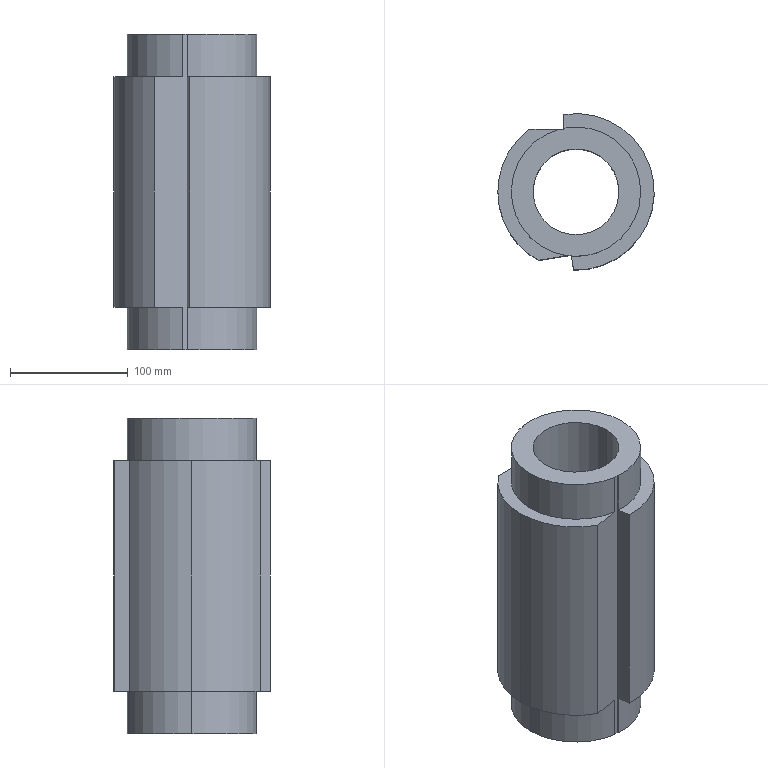Part | SolidWorks | features ICE 2, Extrusion 1 | 1 solid | 21 faces | box 133 x 133 x 268 mm | volume 2196545 mm3 | cylinder 11 | plane 10 | commonest cylinder face diameters 110 x6 133 x3 73 x2
STEP:
#1=CARTESIAN_POINT('',(-7.929,-54.426,36.));
#2=VERTEX_POINT('',#1);
#3=CARTESIAN_POINT('',(-55.,0.,36.));
#4=VERTEX_POINT('',#3);
#5=CARTESIAN_POINT('',(0.,0.,36.));
#6=DIRECTION('',(0.,0.,-1.));
#7=DIRECTION('',(-1.,0.,0.));
#8=AXIS2_PLACEMENT_3D('',#5,#6,#7);
#9=CIRCLE('',#8,55.);
#10=EDGE_CURVE('',#2,#4,#9,.T.);
#11=ORIENTED_EDGE('',*,*,#10,.T.);
#12=CARTESIAN_POINT('',(-55.,0.,0.));
#13=VERTEX_POINT('',#12);
#14=CARTESIAN_POINT('',(-55.,0.,36.));
#15=DIRECTION('',(0.,0.,-1.));
#16=VECTOR('',#15,1000.);
#17=LINE('',#14,#16);
#18=EDGE_CURVE('',#4,#13,#17,.T.);
#19=ORIENTED_EDGE('',*,*,#18,.T.);
#20=CARTESIAN_POINT('',(-7.929,-54.426,0.));
#21=VERTEX_POINT('',#20);
#22=CARTESIAN_POINT('',(0.,0.,0.));
#23=DIRECTION('',(0.,0.,1.));
#24=DIRECTION('',(1.,0.,0.));
#25=AXIS2_PLACEMENT_3D('',#22,#23,#24);
#26=CIRCLE('',#25,55.);
#27=EDGE_CURVE('',#13,#21,#26,.T.);
#28=ORIENTED_EDGE('',*,*,#27,.T.);
#29=CARTESIAN_POINT('',(-7.929,-54.426,36.));
#30=DIRECTION('',(0.,0.,1.));
#31=VECTOR('',#30,1000.);
#32=LINE('',#29,#31);
#33=EDGE_CURVE('',#21,#2,#32,.T.);
#34=ORIENTED_EDGE('',*,*,#33,.T.);
#35=EDGE_LOOP('',(#11,#19,#28,#34));
#36=FACE_OUTER_BOUND('',#35,.T.);
#37=CARTESIAN_POINT('',(0.,0.,36.));
#38=DIRECTION('',(0.,0.,-1.));
#39=DIRECTION('',(-1.,0.,0.));
#40=AXIS2_PLACEMENT_3D('',#37,#38,#39);
#41=CYLINDRICAL_SURFACE('',#40,55.);
#42=ADVANCED_FACE('',(#36),#41,.T.);
#43=CARTESIAN_POINT('',(-3.964,-54.857,232.));
#44=VERTEX_POINT('',#43);
#45=CARTESIAN_POINT('',(55.,0.,232.));
#46=VERTEX_POINT('',#45);
#47=CARTESIAN_POINT('',(0.,0.,232.));
#48=DIRECTION('',(0.,0.,1.));
#49=DIRECTION('',(1.,0.,0.));
#50=AXIS2_PLACEMENT_3D('',#47,#48,#49);
#51=CIRCLE('',#50,55.);
#52=EDGE_CURVE('',#44,#46,#51,.T.);
#53=ORIENTED_EDGE('',*,*,#52,.T.);
#54=CARTESIAN_POINT('',(55.,0.,268.));
#55=VERTEX_POINT('',#54);
#56=CARTESIAN_POINT('',(55.,0.,232.));
#57=DIRECTION('',(0.,0.,1.));
#58=VECTOR('',#57,1000.);
#59=LINE('',#56,#58);
#60=EDGE_CURVE('',#46,#55,#59,.T.);
#61=ORIENTED_EDGE('',*,*,#60,.T.);
#62=CARTESIAN_POINT('',(-3.964,-54.857,268.));
#63=VERTEX_POINT('',#62);
#64=CARTESIAN_POINT('',(0.,0.,268.));
#65=DIRECTION('',(0.,0.,1.));
#66=DIRECTION('',(1.,0.,0.));
#67=AXIS2_PLACEMENT_3D('',#64,#65,#66);
#68=CIRCLE('',#67,55.);
#69=EDGE_CURVE('',#63,#55,#68,.T.);
#70=ORIENTED_EDGE('',*,*,#69,.F.);
#71=CARTESIAN_POINT('',(-3.964,-54.857,232.));
#72=DIRECTION('',(0.,0.,-1.));
#73=VECTOR('',#72,1000.);
#74=LINE('',#71,#73);
#75=EDGE_CURVE('',#63,#44,#74,.T.);
#76=ORIENTED_EDGE('',*,*,#75,.T.);
#77=EDGE_LOOP('',(#53,#61,#70,#76));
#78=FACE_OUTER_BOUND('',#77,.T.);
#79=CARTESIAN_POINT('',(0.,0.,232.));
#80=DIRECTION('',(0.,0.,1.));
#81=DIRECTION('',(1.,0.,0.));
#82=AXIS2_PLACEMENT_3D('',#79,#80,#81);
#83=CYLINDRICAL_SURFACE('',#82,55.);
#84=ADVANCED_FACE('',(#78),#83,.T.);
#85=CARTESIAN_POINT('',(-36.5,0.,268.));
#86=VERTEX_POINT('',#85);
#87=CARTESIAN_POINT('',(36.5,0.,268.));
#88=VERTEX_POINT('',#87);
#89=CARTESIAN_POINT('',(0.,0.,268.));
#90=DIRECTION('',(0.,0.,1.));
#91=DIRECTION('',(1.,0.,0.));
#92=AXIS2_PLACEMENT_3D('',#89,#90,#91);
#93=CIRCLE('',#92,36.5);
#94=EDGE_CURVE('',#86,#88,#93,.T.);
#95=ORIENTED_EDGE('',*,*,#94,.T.);
#96=CARTESIAN_POINT('',(36.5,0.,0.));
#97=VERTEX_POINT('',#96);
#98=CARTESIAN_POINT('',(36.5,0.,268.));
#99=DIRECTION('',(0.,0.,-1.));
#100=VECTOR('',#99,1000.);
#101=LINE('',#98,#100);
#102=EDGE_CURVE('',#88,#97,#101,.T.);
#103=ORIENTED_EDGE('',*,*,#102,.T.);
#104=CARTESIAN_POINT('',(-36.5,0.,0.));
#105=VERTEX_POINT('',#104);
#106=CARTESIAN_POINT('',(0.,0.,0.));
#107=DIRECTION('',(0.,0.,1.));
#108=DIRECTION('',(1.,0.,0.));
#109=AXIS2_PLACEMENT_3D('',#106,#107,#108);
#110=CIRCLE('',#109,36.5);
#111=EDGE_CURVE('',#105,#97,#110,.T.);
#112=ORIENTED_EDGE('',*,*,#111,.F.);
#113=CARTESIAN_POINT('',(-36.5,0.,268.));
#114=DIRECTION('',(0.,0.,-1.));
#115=VECTOR('',#114,1000.);
#116=LINE('',#113,#115);
#117=EDGE_CURVE('',#86,#105,#116,.T.);
#118=ORIENTED_EDGE('',*,*,#117,.F.);
#119=EDGE_LOOP('',(#95,#103,#112,#118));
#120=FACE_OUTER_BOUND('',#119,.T.);
#121=CARTESIAN_POINT('',(0.,0.,268.));
#122=DIRECTION('',(0.,0.,-1.));
#123=DIRECTION('',(-1.,0.,0.));
#124=AXIS2_PLACEMENT_3D('',#121,#122,#123);
#125=CYLINDRICAL_SURFACE('',#124,36.5);
#126=ADVANCED_FACE('',(#120),#125,.F.);
#127=CARTESIAN_POINT('',(-66.5,0.,232.));
#128=VERTEX_POINT('',#127);
#129=CARTESIAN_POINT('',(-32.08,-58.251,232.));
#130=VERTEX_POINT('',#129);
#131=CARTESIAN_POINT('',(0.,0.,232.));
#132=DIRECTION('',(0.,0.,1.));
#133=DIRECTION('',(1.,0.,0.));
#134=AXIS2_PLACEMENT_3D('',#131,#132,#133);
#135=CIRCLE('',#134,66.5);
#136=EDGE_CURVE('',#128,#130,#135,.T.);
#137=ORIENTED_EDGE('',*,*,#136,.F.);
#138=CARTESIAN_POINT('',(-66.5,0.,36.));
#139=VERTEX_POINT('',#138);
#140=CARTESIAN_POINT('',(-66.5,0.,268.));
#141=DIRECTION('',(0.,0.,-1.));
#142=VECTOR('',#141,1000.);
#143=LINE('',#140,#142);
#144=EDGE_CURVE('',#128,#139,#143,.T.);
#145=ORIENTED_EDGE('',*,*,#144,.T.);
#146=CARTESIAN_POINT('',(-32.08,-58.251,36.));
#147=VERTEX_POINT('',#146);
#148=CARTESIAN_POINT('',(0.,0.,36.));
#149=DIRECTION('',(0.,0.,-1.));
#150=DIRECTION('',(-1.,0.,0.));
#151=AXIS2_PLACEMENT_3D('',#148,#149,#150);
#152=CIRCLE('',#151,66.5);
#153=EDGE_CURVE('',#147,#139,#152,.T.);
#154=ORIENTED_EDGE('',*,*,#153,.F.);
#155=CARTESIAN_POINT('',(-32.08,-58.251,268.));
#156=DIRECTION('',(0.,0.,-1.));
#157=VECTOR('',#156,1000.);
#158=LINE('',#155,#157);
#159=EDGE_CURVE('',#130,#147,#158,.T.);
#160=ORIENTED_EDGE('',*,*,#159,.F.);
#161=EDGE_LOOP('',(#137,#145,#154,#160));
#162=FACE_OUTER_BOUND('',#161,.T.);
#163=CARTESIAN_POINT('',(0.,0.,268.));
#164=DIRECTION('',(0.,0.,-1.));
#165=DIRECTION('',(-1.,0.,0.));
#166=AXIS2_PLACEMENT_3D('',#163,#164,#165);
#167=CYLINDRICAL_SURFACE('',#166,66.5);
#168=ADVANCED_FACE('',(#162),#167,.T.);
#169=CARTESIAN_POINT('',(-4.128,-53.824,36.));
#170=DIRECTION('',(-0.9877,-0.1564,0.));
#171=VECTOR('',#170,1000.);
#172=LINE('',#169,#171);
#173=EDGE_CURVE('',#2,#147,#172,.T.);
#174=ORIENTED_EDGE('',*,*,#173,.F.);
#175=ORIENTED_EDGE('',*,*,#33,.F.);
#176=CARTESIAN_POINT('',(-4.128,-53.824,0.));
#177=VERTEX_POINT('',#176);
#178=CARTESIAN_POINT('',(-4.128,-53.824,0.));
#179=DIRECTION('',(0.9877,0.1564,0.));
#180=VECTOR('',#179,1000.);
#181=LINE('',#178,#180);
#182=EDGE_CURVE('',#21,#177,#181,.T.);
#183=ORIENTED_EDGE('',*,*,#182,.T.);
#184=CARTESIAN_POINT('',(-4.128,-53.824,268.));
#185=VERTEX_POINT('',#184);
#186=CARTESIAN_POINT('',(-4.128,-53.824,268.));
#187=DIRECTION('',(0.,0.,-1.));
#188=VECTOR('',#187,1000.);
#189=LINE('',#186,#188);
#190=EDGE_CURVE('',#185,#177,#189,.T.);
#191=ORIENTED_EDGE('',*,*,#190,.F.);
#192=CARTESIAN_POINT('',(-7.929,-54.426,268.));
#193=VERTEX_POINT('',#192);
#194=CARTESIAN_POINT('',(-4.128,-53.824,268.));
#195=DIRECTION('',(0.9877,0.1564,0.));
#196=VECTOR('',#195,1000.);
#197=LINE('',#194,#196);
#198=EDGE_CURVE('',#193,#185,#197,.T.);
#199=ORIENTED_EDGE('',*,*,#198,.F.);
#200=CARTESIAN_POINT('',(-7.929,-54.426,232.));
#201=VERTEX_POINT('',#200);
#202=CARTESIAN_POINT('',(-7.929,-54.426,232.));
#203=DIRECTION('',(0.,0.,1.));
#204=VECTOR('',#203,1000.);
#205=LINE('',#202,#204);
#206=EDGE_CURVE('',#201,#193,#205,.T.);
#207=ORIENTED_EDGE('',*,*,#206,.F.);
#208=CARTESIAN_POINT('',(-4.128,-53.824,232.));
#209=DIRECTION('',(0.9877,0.1564,0.));
#210=VECTOR('',#209,1000.);
#211=LINE('',#208,#210);
#212=EDGE_CURVE('',#130,#201,#211,.T.);
#213=ORIENTED_EDGE('',*,*,#212,.F.);
#214=ORIENTED_EDGE('',*,*,#159,.T.);
#215=EDGE_LOOP('',(#174,#175,#183,#191,#199,#207,#213,#214));
#216=FACE_OUTER_BOUND('',#215,.T.);
#217=CARTESIAN_POINT('',(-4.128,-53.824,268.));
#218=DIRECTION('',(-0.1564,0.9877,0.));
#219=DIRECTION('',(-0.9877,-0.1564,0.));
#220=AXIS2_PLACEMENT_3D('',#217,#218,#219);
#221=PLANE('',#220);
#222=ADVANCED_FACE('',(#216),#221,.F.);
#223=CARTESIAN_POINT('',(-2.126,-66.466,36.));
#224=VERTEX_POINT('',#223);
#225=CARTESIAN_POINT('',(-3.964,-54.857,36.));
#226=VERTEX_POINT('',#225);
#227=CARTESIAN_POINT('',(-4.128,-53.824,36.));
#228=DIRECTION('',(-0.1564,0.9877,0.));
#229=VECTOR('',#228,1000.);
#230=LINE('',#227,#229);
#231=EDGE_CURVE('',#224,#226,#230,.T.);
#232=ORIENTED_EDGE('',*,*,#231,.F.);
#233=CARTESIAN_POINT('',(-2.126,-66.466,232.));
#234=VERTEX_POINT('',#233);
#235=CARTESIAN_POINT('',(-2.126,-66.466,268.));
#236=DIRECTION('',(0.,0.,-1.));
#237=VECTOR('',#236,1000.);
#238=LINE('',#235,#237);
#239=EDGE_CURVE('',#234,#224,#238,.T.);
#240=ORIENTED_EDGE('',*,*,#239,.F.);
#241=CARTESIAN_POINT('',(-4.128,-53.824,232.));
#242=DIRECTION('',(0.1564,-0.9877,0.));
#243=VECTOR('',#242,1000.);
#244=LINE('',#241,#243);
#245=EDGE_CURVE('',#44,#234,#244,.T.);
#246=ORIENTED_EDGE('',*,*,#245,.F.);
#247=ORIENTED_EDGE('',*,*,#75,.F.);
#248=CARTESIAN_POINT('',(-4.128,-53.824,268.));
#249=DIRECTION('',(0.1564,-0.9877,0.));
#250=VECTOR('',#249,1000.);
#251=LINE('',#248,#250);
#252=EDGE_CURVE('',#185,#63,#251,.T.);
#253=ORIENTED_EDGE('',*,*,#252,.F.);
#254=ORIENTED_EDGE('',*,*,#190,.T.);
#255=CARTESIAN_POINT('',(-3.964,-54.857,0.));
#256=VERTEX_POINT('',#255);
#257=CARTESIAN_POINT('',(-4.128,-53.824,0.));
#258=DIRECTION('',(0.1564,-0.9877,0.));
#259=VECTOR('',#258,1000.);
#260=LINE('',#257,#259);
#261=EDGE_CURVE('',#177,#256,#260,.T.);
#262=ORIENTED_EDGE('',*,*,#261,.T.);
#263=CARTESIAN_POINT('',(-3.964,-54.857,36.));
#264=DIRECTION('',(0.,0.,-1.));
#265=VECTOR('',#264,1000.);
#266=LINE('',#263,#265);
#267=EDGE_CURVE('',#226,#256,#266,.T.);
#268=ORIENTED_EDGE('',*,*,#267,.F.);
#269=EDGE_LOOP('',(#232,#240,#246,#247,#253,#254,#262,#268));
#270=FACE_OUTER_BOUND('',#269,.T.);
#271=CARTESIAN_POINT('',(-4.128,-53.824,268.));
#272=DIRECTION('',(0.9877,0.1564,0.));
#273=DIRECTION('',(-0.1564,0.9877,0.));
#274=AXIS2_PLACEMENT_3D('',#271,#272,#273);
#275=PLANE('',#274);
#276=ADVANCED_FACE('',(#270),#275,.F.);
#277=CARTESIAN_POINT('',(-10.3,65.697,36.));
#278=VERTEX_POINT('',#277);
#279=CARTESIAN_POINT('',(0.,0.,36.));
#280=DIRECTION('',(0.,0.,-1.));
#281=DIRECTION('',(-1.,0.,0.));
#282=AXIS2_PLACEMENT_3D('',#279,#280,#281);
#283=CIRCLE('',#282,66.5);
#284=EDGE_CURVE('',#278,#224,#283,.T.);
#285=ORIENTED_EDGE('',*,*,#284,.F.);
#286=CARTESIAN_POINT('',(-10.3,65.697,232.));
#287=VERTEX_POINT('',#286);
#288=CARTESIAN_POINT('',(-10.3,65.697,268.));
#289=DIRECTION('',(0.,0.,-1.));
#290=VECTOR('',#289,1000.);
#291=LINE('',#288,#290);
#292=EDGE_CURVE('',#287,#278,#291,.T.);
#293=ORIENTED_EDGE('',*,*,#292,.F.);
#294=CARTESIAN_POINT('',(0.,0.,232.));
#295=DIRECTION('',(0.,0.,1.));
#296=DIRECTION('',(1.,0.,0.));
#297=AXIS2_PLACEMENT_3D('',#294,#295,#296);
#298=CIRCLE('',#297,66.5);
#299=EDGE_CURVE('',#234,#287,#298,.T.);
#300=ORIENTED_EDGE('',*,*,#299,.F.);
#301=ORIENTED_EDGE('',*,*,#239,.T.);
#302=EDGE_LOOP('',(#285,#293,#300,#301));
#303=FACE_OUTER_BOUND('',#302,.T.);
#304=CARTESIAN_POINT('',(0.,0.,268.));
#305=DIRECTION('',(0.,0.,-1.));
#306=DIRECTION('',(-1.,0.,0.));
#307=AXIS2_PLACEMENT_3D('',#304,#305,#306);
#308=CYLINDRICAL_SURFACE('',#307,66.5);
#309=ADVANCED_FACE('',(#303),#308,.T.);
#310=CARTESIAN_POINT('',(-10.3,54.027,36.));
#311=VERTEX_POINT('',#310);
#312=CARTESIAN_POINT('',(-10.3,53.,36.));
#313=DIRECTION('',(0.,1.,0.));
#314=VECTOR('',#313,1000.);
#315=LINE('',#312,#314);
#316=EDGE_CURVE('',#311,#278,#315,.T.);
#317=ORIENTED_EDGE('',*,*,#316,.F.);
#318=CARTESIAN_POINT('',(-10.3,54.027,0.));
#319=VERTEX_POINT('',#318);
#320=CARTESIAN_POINT('',(-10.3,54.027,36.));
#321=DIRECTION('',(0.,0.,1.));
#322=VECTOR('',#321,1000.);
#323=LINE('',#320,#322);
#324=EDGE_CURVE('',#319,#311,#323,.T.);
#325=ORIENTED_EDGE('',*,*,#324,.F.);
#326=CARTESIAN_POINT('',(-10.3,53.,0.));
#327=VERTEX_POINT('',#326);
#328=CARTESIAN_POINT('',(-10.3,53.,0.));
#329=DIRECTION('',(0.,-1.,0.));
#330=VECTOR('',#329,1000.);
#331=LINE('',#328,#330);
#332=EDGE_CURVE('',#319,#327,#331,.T.);
#333=ORIENTED_EDGE('',*,*,#332,.T.);
#334=CARTESIAN_POINT('',(-10.3,53.,268.));
#335=VERTEX_POINT('',#334);
#336=CARTESIAN_POINT('',(-10.3,53.,268.));
#337=DIRECTION('',(0.,0.,-1.));
#338=VECTOR('',#337,1000.);
#339=LINE('',#336,#338);
#340=EDGE_CURVE('',#335,#327,#339,.T.);
#341=ORIENTED_EDGE('',*,*,#340,.F.);
#342=CARTESIAN_POINT('',(-10.3,54.027,268.));
#343=VERTEX_POINT('',#342);
#344=CARTESIAN_POINT('',(-10.3,53.,268.));
#345=DIRECTION('',(0.,-1.,0.));
#346=VECTOR('',#345,1000.);
#347=LINE('',#344,#346);
#348=EDGE_CURVE('',#343,#335,#347,.T.);
#349=ORIENTED_EDGE('',*,*,#348,.F.);
#350=CARTESIAN_POINT('',(-10.3,54.027,232.));
#351=VERTEX_POINT('',#350);
#352=CARTESIAN_POINT('',(-10.3,54.027,232.));
#353=DIRECTION('',(0.,0.,1.));
#354=VECTOR('',#353,1000.);
#355=LINE('',#352,#354);
#356=EDGE_CURVE('',#351,#343,#355,.T.);
#357=ORIENTED_EDGE('',*,*,#356,.F.);
#358=CARTESIAN_POINT('',(-10.3,53.,232.));
#359=DIRECTION('',(0.,-1.,0.));
#360=VECTOR('',#359,1000.);
#361=LINE('',#358,#360);
#362=EDGE_CURVE('',#287,#351,#361,.T.);
#363=ORIENTED_EDGE('',*,*,#362,.F.);
#364=ORIENTED_EDGE('',*,*,#292,.T.);
#365=EDGE_LOOP('',(#317,#325,#333,#341,#349,#357,#363,#364));
#366=FACE_OUTER_BOUND('',#365,.T.);
#367=CARTESIAN_POINT('',(-10.3,53.,268.));
#368=DIRECTION('',(1.,0.,0.));
#369=DIRECTION('',(0.,0.,-1.));
#370=AXIS2_PLACEMENT_3D('',#367,#368,#369);
#371=PLANE('',#370);
#372=ADVANCED_FACE('',(#366),#371,.F.);
#373=CARTESIAN_POINT('',(-40.165,53.,36.));
#374=VERTEX_POINT('',#373);
#375=CARTESIAN_POINT('',(-14.697,53.,36.));
#376=VERTEX_POINT('',#375);
#377=CARTESIAN_POINT('',(-40.165,53.,36.));
#378=DIRECTION('',(1.,0.,0.));
#379=VECTOR('',#378,1000.);
#380=LINE('',#377,#379);
#381=EDGE_CURVE('',#374,#376,#380,.T.);
#382=ORIENTED_EDGE('',*,*,#381,.F.);
#383=CARTESIAN_POINT('',(-40.165,53.,232.));
#384=VERTEX_POINT('',#383);
#385=CARTESIAN_POINT('',(-40.165,53.,268.));
#386=DIRECTION('',(0.,0.,-1.));
#387=VECTOR('',#386,1000.);
#388=LINE('',#385,#387);
#389=EDGE_CURVE('',#384,#374,#388,.T.);
#390=ORIENTED_EDGE('',*,*,#389,.F.);
#391=CARTESIAN_POINT('',(-14.697,53.,232.));
#392=VERTEX_POINT('',#391);
#393=CARTESIAN_POINT('',(-40.165,53.,232.));
#394=DIRECTION('',(-1.,0.,0.));
#395=VECTOR('',#394,1000.);
#396=LINE('',#393,#395);
#397=EDGE_CURVE('',#392,#384,#396,.T.);
#398=ORIENTED_EDGE('',*,*,#397,.F.);
#399=CARTESIAN_POINT('',(-14.697,53.,268.));
#400=VERTEX_POINT('',#399);
#401=CARTESIAN_POINT('',(-14.697,53.,232.));
#402=DIRECTION('',(0.,0.,-1.));
#403=VECTOR('',#402,1000.);
#404=LINE('',#401,#403);
#405=EDGE_CURVE('',#400,#392,#404,.T.);
#406=ORIENTED_EDGE('',*,*,#405,.F.);
#407=CARTESIAN_POINT('',(-40.165,53.,268.));
#408=DIRECTION('',(-1.,0.,0.));
#409=VECTOR('',#408,1000.);
#410=LINE('',#407,#409);
#411=EDGE_CURVE('',#335,#400,#410,.T.);
#412=ORIENTED_EDGE('',*,*,#411,.F.);
#413=ORIENTED_EDGE('',*,*,#340,.T.);
#414=CARTESIAN_POINT('',(-14.697,53.,0.));
#415=VERTEX_POINT('',#414);
#416=CARTESIAN_POINT('',(-40.165,53.,0.));
#417=DIRECTION('',(-1.,0.,0.));
#418=VECTOR('',#417,1000.);
#419=LINE('',#416,#418);
#420=EDGE_CURVE('',#327,#415,#419,.T.);
#421=ORIENTED_EDGE('',*,*,#420,.T.);
#422=CARTESIAN_POINT('',(-14.697,53.,36.));
#423=DIRECTION('',(0.,0.,-1.));
#424=VECTOR('',#423,1000.);
#425=LINE('',#422,#424);
#426=EDGE_CURVE('',#376,#415,#425,.T.);
#427=ORIENTED_EDGE('',*,*,#426,.F.);
#428=EDGE_LOOP('',(#382,#390,#398,#406,#412,#413,#421,#427));
#429=FACE_OUTER_BOUND('',#428,.T.);
#430=CARTESIAN_POINT('',(-40.165,53.,268.));
#431=DIRECTION('',(0.,-1.,0.));
#432=DIRECTION('',(0.,0.,-1.));
#433=AXIS2_PLACEMENT_3D('',#430,#431,#432);
#434=PLANE('',#433);
#435=ADVANCED_FACE('',(#429),#434,.F.);
#436=ORIENTED_EDGE('',*,*,#144,.F.);
#437=CARTESIAN_POINT('',(0.,0.,232.));
#438=DIRECTION('',(0.,0.,1.));
#439=DIRECTION('',(1.,0.,0.));
#440=AXIS2_PLACEMENT_3D('',#437,#438,#439);
#441=CIRCLE('',#440,66.5);
#442=EDGE_CURVE('',#384,#128,#441,.T.);
#443=ORIENTED_EDGE('',*,*,#442,.F.);
#444=ORIENTED_EDGE('',*,*,#389,.T.);
#445=CARTESIAN_POINT('',(0.,0.,36.));
#446=DIRECTION('',(0.,0.,-1.));
#447=DIRECTION('',(-1.,0.,0.));
#448=AXIS2_PLACEMENT_3D('',#445,#446,#447);
#449=CIRCLE('',#448,66.5);
#450=EDGE_CURVE('',#139,#374,#449,.T.);
#451=ORIENTED_EDGE('',*,*,#450,.F.);
#452=EDGE_LOOP('',(#436,#443,#444,#451));
#453=FACE_OUTER_BOUND('',#452,.T.);
#454=CARTESIAN_POINT('',(0.,0.,268.));
#455=DIRECTION('',(0.,0.,-1.));
#456=DIRECTION('',(-1.,0.,0.));
#457=AXIS2_PLACEMENT_3D('',#454,#455,#456);
#458=CYLINDRICAL_SURFACE('',#457,66.5);
#459=ADVANCED_FACE('',(#453),#458,.T.);
#460=ORIENTED_EDGE('',*,*,#111,.T.);
#461=CARTESIAN_POINT('',(0.,0.,0.));
#462=DIRECTION('',(0.,0.,1.));
#463=DIRECTION('',(1.,0.,0.));
#464=AXIS2_PLACEMENT_3D('',#461,#462,#463);
#465=CIRCLE('',#464,36.5);
#466=EDGE_CURVE('',#97,#105,#465,.T.);
#467=ORIENTED_EDGE('',*,*,#466,.T.);
#468=EDGE_LOOP('',(#460,#467));
#469=FACE_BOUND('',#468,.T.);
#470=CARTESIAN_POINT('',(0.,0.,0.));
#471=DIRECTION('',(0.,0.,1.));
#472=DIRECTION('',(1.,0.,0.));
#473=AXIS2_PLACEMENT_3D('',#470,#471,#472);
#474=CIRCLE('',#473,55.);
#475=EDGE_CURVE('',#415,#13,#474,.T.);
#476=ORIENTED_EDGE('',*,*,#475,.F.);
#477=ORIENTED_EDGE('',*,*,#420,.F.);
#478=ORIENTED_EDGE('',*,*,#332,.F.);
#479=CARTESIAN_POINT('',(0.,0.,0.));
#480=DIRECTION('',(0.,0.,1.));
#481=DIRECTION('',(1.,0.,0.));
#482=AXIS2_PLACEMENT_3D('',#479,#480,#481);
#483=CIRCLE('',#482,55.);
#484=EDGE_CURVE('',#256,#319,#483,.T.);
#485=ORIENTED_EDGE('',*,*,#484,.F.);
#486=ORIENTED_EDGE('',*,*,#261,.F.);
#487=ORIENTED_EDGE('',*,*,#182,.F.);
#488=ORIENTED_EDGE('',*,*,#27,.F.);
#489=EDGE_LOOP('',(#476,#477,#478,#485,#486,#487,#488));
#490=FACE_OUTER_BOUND('',#489,.T.);
#491=CARTESIAN_POINT('',(0.,0.,0.));
#492=DIRECTION('',(0.,0.,1.));
#493=DIRECTION('',(1.,0.,0.));
#494=AXIS2_PLACEMENT_3D('',#491,#492,#493);
#495=PLANE('',#494);
#496=ADVANCED_FACE('',(#469,#490),#495,.F.);
#497=ORIENTED_EDGE('',*,*,#94,.F.);
#498=CARTESIAN_POINT('',(0.,0.,268.));
#499=DIRECTION('',(0.,0.,1.));
#500=DIRECTION('',(1.,0.,0.));
#501=AXIS2_PLACEMENT_3D('',#498,#499,#500);
#502=CIRCLE('',#501,36.5);
#503=EDGE_CURVE('',#88,#86,#502,.T.);
#504=ORIENTED_EDGE('',*,*,#503,.F.);
#505=EDGE_LOOP('',(#497,#504));
#506=FACE_BOUND('',#505,.T.);
#507=ORIENTED_EDGE('',*,*,#411,.T.);
#508=CARTESIAN_POINT('',(0.,0.,268.));
#509=DIRECTION('',(0.,0.,1.));
#510=DIRECTION('',(1.,0.,0.));
#511=AXIS2_PLACEMENT_3D('',#508,#509,#510);
#512=CIRCLE('',#511,55.);
#513=EDGE_CURVE('',#400,#193,#512,.T.);
#514=ORIENTED_EDGE('',*,*,#513,.T.);
#515=ORIENTED_EDGE('',*,*,#198,.T.);
#516=ORIENTED_EDGE('',*,*,#252,.T.);
#517=ORIENTED_EDGE('',*,*,#69,.T.);
#518=CARTESIAN_POINT('',(0.,0.,268.));
#519=DIRECTION('',(0.,0.,1.));
#520=DIRECTION('',(1.,0.,0.));
#521=AXIS2_PLACEMENT_3D('',#518,#519,#520);
#522=CIRCLE('',#521,55.);
#523=EDGE_CURVE('',#55,#343,#522,.T.);
#524=ORIENTED_EDGE('',*,*,#523,.T.);
#525=ORIENTED_EDGE('',*,*,#348,.T.);
#526=EDGE_LOOP('',(#507,#514,#515,#516,#517,#524,#525));
#527=FACE_OUTER_BOUND('',#526,.T.);
#528=CARTESIAN_POINT('',(0.,0.,268.));
#529=DIRECTION('',(0.,0.,1.));
#530=DIRECTION('',(1.,0.,0.));
#531=AXIS2_PLACEMENT_3D('',#528,#529,#530);
#532=PLANE('',#531);
#533=ADVANCED_FACE('',(#506,#527),#532,.T.);
#534=ORIENTED_EDGE('',*,*,#102,.F.);
#535=ORIENTED_EDGE('',*,*,#503,.T.);
#536=ORIENTED_EDGE('',*,*,#117,.T.);
#537=ORIENTED_EDGE('',*,*,#466,.F.);
#538=EDGE_LOOP('',(#534,#535,#536,#537));
#539=FACE_OUTER_BOUND('',#538,.T.);
#540=CARTESIAN_POINT('',(0.,0.,268.));
#541=DIRECTION('',(0.,0.,-1.));
#542=DIRECTION('',(-1.,0.,0.));
#543=AXIS2_PLACEMENT_3D('',#540,#541,#542);
#544=CYLINDRICAL_SURFACE('',#543,36.5);
#545=ADVANCED_FACE('',(#539),#544,.F.);
#546=ORIENTED_EDGE('',*,*,#212,.T.);
#547=CARTESIAN_POINT('',(0.,0.,232.));
#548=DIRECTION('',(0.,0.,1.));
#549=DIRECTION('',(1.,0.,0.));
#550=AXIS2_PLACEMENT_3D('',#547,#548,#549);
#551=CIRCLE('',#550,55.);
#552=EDGE_CURVE('',#392,#201,#551,.T.);
#553=ORIENTED_EDGE('',*,*,#552,.F.);
#554=ORIENTED_EDGE('',*,*,#397,.T.);
#555=ORIENTED_EDGE('',*,*,#442,.T.);
#556=ORIENTED_EDGE('',*,*,#136,.T.);
#557=EDGE_LOOP('',(#546,#553,#554,#555,#556));
#558=FACE_OUTER_BOUND('',#557,.T.);
#559=CARTESIAN_POINT('',(0.,0.,232.));
#560=DIRECTION('',(0.,0.,1.));
#561=DIRECTION('',(1.,0.,0.));
#562=AXIS2_PLACEMENT_3D('',#559,#560,#561);
#563=PLANE('',#562);
#564=ADVANCED_FACE('',(#558),#563,.T.);
#565=ORIENTED_EDGE('',*,*,#206,.T.);
#566=ORIENTED_EDGE('',*,*,#513,.F.);
#567=ORIENTED_EDGE('',*,*,#405,.T.);
#568=ORIENTED_EDGE('',*,*,#552,.T.);
#569=EDGE_LOOP('',(#565,#566,#567,#568));
#570=FACE_OUTER_BOUND('',#569,.T.);
#571=CARTESIAN_POINT('',(0.,0.,232.));
#572=DIRECTION('',(0.,0.,1.));
#573=DIRECTION('',(1.,0.,0.));
#574=AXIS2_PLACEMENT_3D('',#571,#572,#573);
#575=CYLINDRICAL_SURFACE('',#574,55.);
#576=ADVANCED_FACE('',(#570),#575,.T.);
#577=ORIENTED_EDGE('',*,*,#60,.F.);
#578=CARTESIAN_POINT('',(0.,0.,232.));
#579=DIRECTION('',(0.,0.,1.));
#580=DIRECTION('',(1.,0.,0.));
#581=AXIS2_PLACEMENT_3D('',#578,#579,#580);
#582=CIRCLE('',#581,55.);
#583=EDGE_CURVE('',#46,#351,#582,.T.);
#584=ORIENTED_EDGE('',*,*,#583,.T.);
#585=ORIENTED_EDGE('',*,*,#356,.T.);
#586=ORIENTED_EDGE('',*,*,#523,.F.);
#587=EDGE_LOOP('',(#577,#584,#585,#586));
#588=FACE_OUTER_BOUND('',#587,.T.);
#589=CARTESIAN_POINT('',(0.,0.,232.));
#590=DIRECTION('',(0.,0.,1.));
#591=DIRECTION('',(1.,0.,0.));
#592=AXIS2_PLACEMENT_3D('',#589,#590,#591);
#593=CYLINDRICAL_SURFACE('',#592,55.);
#594=ADVANCED_FACE('',(#588),#593,.T.);
#595=ORIENTED_EDGE('',*,*,#245,.T.);
#596=ORIENTED_EDGE('',*,*,#299,.T.);
#597=ORIENTED_EDGE('',*,*,#362,.T.);
#598=ORIENTED_EDGE('',*,*,#583,.F.);
#599=ORIENTED_EDGE('',*,*,#52,.F.);
#600=EDGE_LOOP('',(#595,#596,#597,#598,#599));
#601=FACE_OUTER_BOUND('',#600,.T.);
#602=CARTESIAN_POINT('',(0.,0.,232.));
#603=DIRECTION('',(0.,0.,1.));
#604=DIRECTION('',(1.,0.,0.));
#605=AXIS2_PLACEMENT_3D('',#602,#603,#604);
#606=PLANE('',#605);
#607=ADVANCED_FACE('',(#601),#606,.T.);
#608=ORIENTED_EDGE('',*,*,#267,.T.);
#609=ORIENTED_EDGE('',*,*,#484,.T.);
#610=ORIENTED_EDGE('',*,*,#324,.T.);
#611=CARTESIAN_POINT('',(0.,0.,36.));
#612=DIRECTION('',(0.,0.,-1.));
#613=DIRECTION('',(-1.,0.,0.));
#614=AXIS2_PLACEMENT_3D('',#611,#612,#613);
#615=CIRCLE('',#614,55.);
#616=EDGE_CURVE('',#311,#226,#615,.T.);
#617=ORIENTED_EDGE('',*,*,#616,.T.);
#618=EDGE_LOOP('',(#608,#609,#610,#617));
#619=FACE_OUTER_BOUND('',#618,.T.);
#620=CARTESIAN_POINT('',(0.,0.,36.));
#621=DIRECTION('',(0.,0.,-1.));
#622=DIRECTION('',(-1.,0.,0.));
#623=AXIS2_PLACEMENT_3D('',#620,#621,#622);
#624=CYLINDRICAL_SURFACE('',#623,55.);
#625=ADVANCED_FACE('',(#619),#624,.T.);
#626=ORIENTED_EDGE('',*,*,#231,.T.);
#627=ORIENTED_EDGE('',*,*,#616,.F.);
#628=ORIENTED_EDGE('',*,*,#316,.T.);
#629=ORIENTED_EDGE('',*,*,#284,.T.);
#630=EDGE_LOOP('',(#626,#627,#628,#629));
#631=FACE_OUTER_BOUND('',#630,.T.);
#632=CARTESIAN_POINT('',(0.,0.,36.));
#633=DIRECTION('',(0.,0.,-1.));
#634=DIRECTION('',(-1.,0.,0.));
#635=AXIS2_PLACEMENT_3D('',#632,#633,#634);
#636=PLANE('',#635);
#637=ADVANCED_FACE('',(#631),#636,.T.);
#638=ORIENTED_EDGE('',*,*,#173,.T.);
#639=ORIENTED_EDGE('',*,*,#153,.T.);
#640=ORIENTED_EDGE('',*,*,#450,.T.);
#641=ORIENTED_EDGE('',*,*,#381,.T.);
#642=CARTESIAN_POINT('',(0.,0.,36.));
#643=DIRECTION('',(0.,0.,-1.));
#644=DIRECTION('',(-1.,0.,0.));
#645=AXIS2_PLACEMENT_3D('',#642,#643,#644);
#646=CIRCLE('',#645,55.);
#647=EDGE_CURVE('',#4,#376,#646,.T.);
#648=ORIENTED_EDGE('',*,*,#647,.F.);
#649=ORIENTED_EDGE('',*,*,#10,.F.);
#650=EDGE_LOOP('',(#638,#639,#640,#641,#648,#649));
#651=FACE_OUTER_BOUND('',#650,.T.);
#652=CARTESIAN_POINT('',(0.,0.,36.));
#653=DIRECTION('',(0.,0.,-1.));
#654=DIRECTION('',(-1.,0.,0.));
#655=AXIS2_PLACEMENT_3D('',#652,#653,#654);
#656=PLANE('',#655);
#657=ADVANCED_FACE('',(#651),#656,.T.);
#658=ORIENTED_EDGE('',*,*,#18,.F.);
#659=ORIENTED_EDGE('',*,*,#647,.T.);
#660=ORIENTED_EDGE('',*,*,#426,.T.);
#661=ORIENTED_EDGE('',*,*,#475,.T.);
#662=EDGE_LOOP('',(#658,#659,#660,#661));
#663=FACE_OUTER_BOUND('',#662,.T.);
#664=CARTESIAN_POINT('',(0.,0.,36.));
#665=DIRECTION('',(0.,0.,-1.));
#666=DIRECTION('',(-1.,0.,0.));
#667=AXIS2_PLACEMENT_3D('',#664,#665,#666);
#668=CYLINDRICAL_SURFACE('',#667,55.);
#669=ADVANCED_FACE('',(#663),#668,.T.);
#670=CLOSED_SHELL('',(#42,#84,#126,#168,#222,#276,#309,#372,#435,#459,#496,#533,#545,#564,#576,#594,#607,#625,#637,#657,#669));
#671=MANIFOLD_SOLID_BREP('',#670);
#672=CARTESIAN_POINT('',(0.,0.,0.));
#673=DIRECTION('',(0.,0.,1.));
#674=DIRECTION('',(1.,0.,0.));
#675=AXIS2_PLACEMENT_3D('',#672,#673,#674);
#676=(LENGTH_UNIT()NAMED_UNIT(*)SI_UNIT(.MILLI.,.METRE.));
#677=UNCERTAINTY_MEASURE_WITH_UNIT(LENGTH_MEASURE(0.00001),#676,'','');
#678=(NAMED_UNIT(*)PLANE_ANGLE_UNIT()SI_UNIT($,.RADIAN.));
#679=(NAMED_UNIT(*)SI_UNIT($,.STERADIAN.)SOLID_ANGLE_UNIT());
#680=(GEOMETRIC_REPRESENTATION_CONTEXT(3)GLOBAL_UNCERTAINTY_ASSIGNED_CONTEXT((#677))GLOBAL_UNIT_ASSIGNED_CONTEXT((#676,#678,#679))REPRESENTATION_CONTEXT('',''));
#681=ADVANCED_BREP_SHAPE_REPRESENTATION('',(#671,#675),#680);